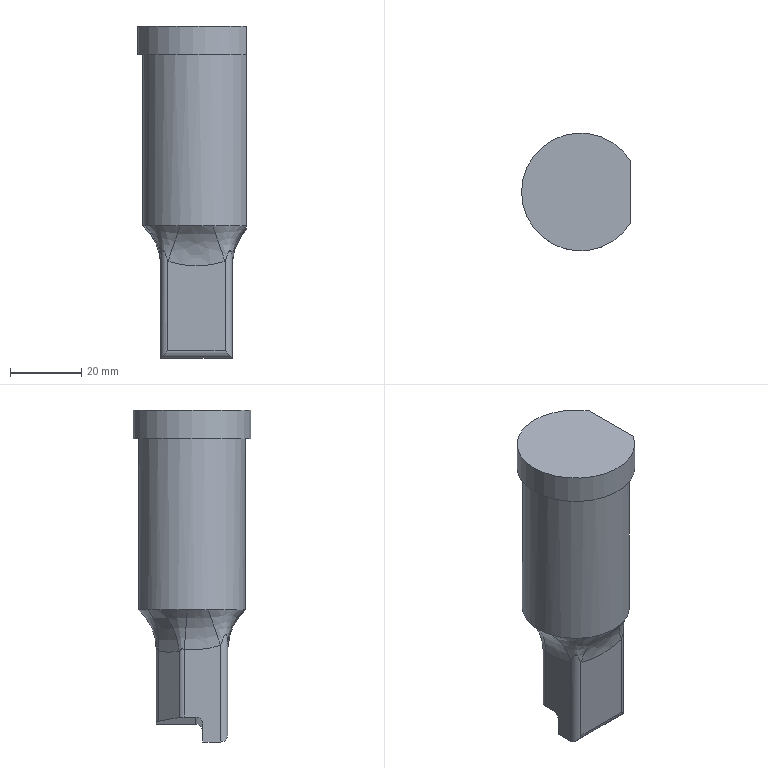Part | NX | features solid 2 | 1 solid | 34 faces | box 30.786 x 33 x 93 mm | volume 53674 mm3 | plane 13 | cylinder 11 | spline 10 | commonest cylinder face diameters 4 x9 30 x1 33 x1
STEP:
#1=CARTESIAN_POINT('',(187.901,-184.385,22.));
#2=VERTEX_POINT('',#1);
#3=CARTESIAN_POINT('',(187.901,-184.385,70.));
#4=VERTEX_POINT('',#3);
#5=CARTESIAN_POINT('',(187.901,-184.385,-33.));
#6=DIRECTION('',(0.,0.,1.));
#7=VECTOR('',#6,1000.);
#8=LINE('',#5,#7);
#9=EDGE_CURVE('',#2,#4,#8,.T.);
#10=ORIENTED_EDGE('',*,*,#9,.T.);
#11=CARTESIAN_POINT('',(187.901,-173.615,70.));
#12=VERTEX_POINT('',#11);
#13=CARTESIAN_POINT('',(173.901,-179.,70.));
#14=DIRECTION('',(0.,0.,1.));
#15=DIRECTION('',(1.,0.,0.));
#16=AXIS2_PLACEMENT_3D('',#13,#14,#15);
#17=CIRCLE('',#16,15.);
#18=EDGE_CURVE('',#4,#12,#17,.F.);
#19=ORIENTED_EDGE('',*,*,#18,.T.);
#20=CARTESIAN_POINT('',(187.901,-173.615,22.));
#21=VERTEX_POINT('',#20);
#22=CARTESIAN_POINT('',(187.901,-173.615,-33.));
#23=DIRECTION('',(0.,0.,1.));
#24=VECTOR('',#23,1000.);
#25=LINE('',#22,#24);
#26=EDGE_CURVE('',#12,#21,#25,.F.);
#27=ORIENTED_EDGE('',*,*,#26,.T.);
#28=CARTESIAN_POINT('',(178.472,-164.714,22.));
#29=VERTEX_POINT('',#28);
#30=CARTESIAN_POINT('',(173.901,-179.,22.));
#31=DIRECTION('',(0.,0.,1.));
#32=DIRECTION('',(1.,0.,0.));
#33=AXIS2_PLACEMENT_3D('',#30,#31,#32);
#34=CIRCLE('',#33,15.);
#35=EDGE_CURVE('',#21,#29,#34,.T.);
#36=ORIENTED_EDGE('',*,*,#35,.T.);
#37=CARTESIAN_POINT('',(172.603,-164.056,22.));
#38=VERTEX_POINT('',#37);
#39=CARTESIAN_POINT('',(173.901,-179.,22.));
#40=DIRECTION('',(0.,0.,1.));
#41=DIRECTION('',(1.,0.,0.));
#42=AXIS2_PLACEMENT_3D('',#39,#40,#41);
#43=CIRCLE('',#42,15.);
#44=EDGE_CURVE('',#29,#38,#43,.T.);
#45=ORIENTED_EDGE('',*,*,#44,.T.);
#46=CARTESIAN_POINT('',(165.226,-166.763,22.));
#47=VERTEX_POINT('',#46);
#48=CARTESIAN_POINT('',(173.901,-179.,22.));
#49=DIRECTION('',(0.,0.,1.));
#50=DIRECTION('',(1.,0.,0.));
#51=AXIS2_PLACEMENT_3D('',#48,#49,#50);
#52=CIRCLE('',#51,15.);
#53=EDGE_CURVE('',#38,#47,#52,.T.);
#54=ORIENTED_EDGE('',*,*,#53,.T.);
#55=CARTESIAN_POINT('',(161.663,-170.325,22.));
#56=VERTEX_POINT('',#55);
#57=CARTESIAN_POINT('',(173.901,-179.,22.));
#58=DIRECTION('',(0.,0.,1.));
#59=DIRECTION('',(1.,0.,0.));
#60=AXIS2_PLACEMENT_3D('',#57,#58,#59);
#61=CIRCLE('',#60,15.);
#62=EDGE_CURVE('',#47,#56,#61,.T.);
#63=ORIENTED_EDGE('',*,*,#62,.T.);
#64=CARTESIAN_POINT('',(158.957,-177.702,22.));
#65=VERTEX_POINT('',#64);
#66=CARTESIAN_POINT('',(173.901,-179.,22.));
#67=DIRECTION('',(0.,0.,1.));
#68=DIRECTION('',(1.,0.,0.));
#69=AXIS2_PLACEMENT_3D('',#66,#67,#68);
#70=CIRCLE('',#69,15.);
#71=EDGE_CURVE('',#56,#65,#70,.T.);
#72=ORIENTED_EDGE('',*,*,#71,.T.);
#73=CARTESIAN_POINT('',(159.614,-183.572,22.));
#74=VERTEX_POINT('',#73);
#75=CARTESIAN_POINT('',(173.901,-179.,22.));
#76=DIRECTION('',(0.,0.,1.));
#77=DIRECTION('',(1.,0.,0.));
#78=AXIS2_PLACEMENT_3D('',#75,#76,#77);
#79=CIRCLE('',#78,15.);
#80=EDGE_CURVE('',#65,#74,#79,.T.);
#81=ORIENTED_EDGE('',*,*,#80,.T.);
#82=CARTESIAN_POINT('',(169.329,-193.286,22.));
#83=VERTEX_POINT('',#82);
#84=CARTESIAN_POINT('',(173.901,-179.,22.));
#85=DIRECTION('',(0.,0.,1.));
#86=DIRECTION('',(1.,0.,0.));
#87=AXIS2_PLACEMENT_3D('',#84,#85,#86);
#88=CIRCLE('',#87,15.);
#89=EDGE_CURVE('',#74,#83,#88,.T.);
#90=ORIENTED_EDGE('',*,*,#89,.T.);
#91=CARTESIAN_POINT('',(178.472,-193.286,22.));
#92=VERTEX_POINT('',#91);
#93=CARTESIAN_POINT('',(173.901,-179.,22.));
#94=DIRECTION('',(0.,0.,1.));
#95=DIRECTION('',(1.,0.,0.));
#96=AXIS2_PLACEMENT_3D('',#93,#94,#95);
#97=CIRCLE('',#96,15.);
#98=EDGE_CURVE('',#83,#92,#97,.T.);
#99=ORIENTED_EDGE('',*,*,#98,.T.);
#100=CARTESIAN_POINT('',(173.901,-179.,22.));
#101=DIRECTION('',(0.,0.,1.));
#102=DIRECTION('',(1.,0.,0.));
#103=AXIS2_PLACEMENT_3D('',#100,#101,#102);
#104=CIRCLE('',#103,15.);
#105=EDGE_CURVE('',#92,#2,#104,.T.);
#106=ORIENTED_EDGE('',*,*,#105,.T.);
#107=EDGE_LOOP('',(#10,#19,#27,#36,#45,#54,#63,#72,#81,#90,#99,#106));
#108=FACE_BOUND('',#107,.T.);
#109=CARTESIAN_POINT('',(173.901,-179.,-33.));
#110=DIRECTION('',(0.,0.,1.));
#111=DIRECTION('',(1.,0.,0.));
#112=AXIS2_PLACEMENT_3D('',#109,#110,#111);
#113=CYLINDRICAL_SURFACE('',#112,15.);
#114=ADVANCED_FACE('',(#108),#113,.T.);
#115=CARTESIAN_POINT('',(174.401,-169.,-10.));
#116=VERTEX_POINT('',#115);
#117=CARTESIAN_POINT('',(174.901,-169.,-10.));
#118=VERTEX_POINT('',#117);
#119=CARTESIAN_POINT('',(171.729,-169.,-10.));
#120=DIRECTION('',(1.,0.,0.));
#121=VECTOR('',#120,1000.);
#122=LINE('',#119,#121);
#123=EDGE_CURVE('',#116,#118,#122,.T.);
#124=ORIENTED_EDGE('',*,*,#123,.F.);
#125=CARTESIAN_POINT('',(171.729,-169.,-9.491));
#126=VERTEX_POINT('',#125);
#127=CARTESIAN_POINT('',(174.401,-169.,-10.));
#128=DIRECTION('',(-0.9823,0.,0.1871));
#129=VECTOR('',#128,1000.);
#130=LINE('',#127,#129);
#131=EDGE_CURVE('',#116,#126,#130,.T.);
#132=ORIENTED_EDGE('',*,*,#131,.T.);
#133=CARTESIAN_POINT('',(171.729,-169.,10.905));
#134=VERTEX_POINT('',#133);
#135=CARTESIAN_POINT('',(171.729,-169.,-64.));
#136=DIRECTION('',(0.,0.,1.));
#137=VECTOR('',#136,1000.);
#138=LINE('',#135,#137);
#139=EDGE_CURVE('',#126,#134,#138,.T.);
#140=ORIENTED_EDGE('',*,*,#139,.T.);
#141=CARTESIAN_POINT('',(181.901,-169.,12.077));
#142=VERTEX_POINT('',#141);
#143=CARTESIAN_POINT('',(171.729,-169.,10.905));
#144=CARTESIAN_POINT('',(173.434,-169.,10.77));
#145=CARTESIAN_POINT('',(176.026,-169.,10.807));
#146=CARTESIAN_POINT('',(179.4,-169.,11.334));
#147=CARTESIAN_POINT('',(181.107,-169.,11.803));
#148=CARTESIAN_POINT('',(181.901,-169.,12.077));
#149=B_SPLINE_CURVE_WITH_KNOTS('',3,(#143,#144,#145,#146,#147,#148),.UNSPECIFIED.,.F.,.F.,(4,1,1,4),(0.,0.5,0.75,1.),.UNSPECIFIED.);
#150=EDGE_CURVE('',#134,#142,#149,.T.);
#151=ORIENTED_EDGE('',*,*,#150,.T.);
#152=CARTESIAN_POINT('',(181.901,-169.,-8.444));
#153=VERTEX_POINT('',#152);
#154=CARTESIAN_POINT('',(181.901,-169.,-64.));
#155=DIRECTION('',(0.,0.,1.));
#156=VECTOR('',#155,1000.);
#157=LINE('',#154,#156);
#158=EDGE_CURVE('',#153,#142,#157,.T.);
#159=ORIENTED_EDGE('',*,*,#158,.F.);
#160=CARTESIAN_POINT('',(174.901,-169.,-10.));
#161=DIRECTION('',(-0.9762,0.,-0.2169));
#162=VECTOR('',#161,1000.);
#163=LINE('',#160,#162);
#164=EDGE_CURVE('',#153,#118,#163,.T.);
#165=ORIENTED_EDGE('',*,*,#164,.T.);
#166=EDGE_LOOP('',(#124,#132,#140,#151,#159,#165));
#167=FACE_BOUND('',#166,.T.);
#168=CARTESIAN_POINT('',(171.729,-169.,-64.));
#169=DIRECTION('',(0.,-1.,0.));
#170=DIRECTION('',(1.,0.,0.));
#171=AXIS2_PLACEMENT_3D('',#168,#169,#170);
#172=PLANE('',#171);
#173=ADVANCED_FACE('',(#167),#172,.F.);
#174=CARTESIAN_POINT('',(183.901,-171.,-8.));
#175=VERTEX_POINT('',#174);
#176=CARTESIAN_POINT('',(183.901,-171.,12.077));
#177=VERTEX_POINT('',#176);
#178=CARTESIAN_POINT('',(183.901,-171.,-64.));
#179=DIRECTION('',(0.,0.,1.));
#180=VECTOR('',#179,1000.);
#181=LINE('',#178,#180);
#182=EDGE_CURVE('',#175,#177,#181,.T.);
#183=ORIENTED_EDGE('',*,*,#182,.F.);
#184=CARTESIAN_POINT('',(181.901,-171.,-8.444));
#185=DIRECTION('',(0.2169,0.,-0.9762));
#186=DIRECTION('',(0.9762,0.,0.2169));
#187=AXIS2_PLACEMENT_3D('',#184,#185,#186);
#188=ELLIPSE('',#187,2.049,2.);
#189=EDGE_CURVE('',#175,#153,#188,.F.);
#190=ORIENTED_EDGE('',*,*,#189,.T.);
#191=ORIENTED_EDGE('',*,*,#158,.T.);
#192=CARTESIAN_POINT('',(181.901,-169.,12.077));
#193=CARTESIAN_POINT('',(182.018,-169.,12.421));
#194=CARTESIAN_POINT('',(182.214,-169.021,12.984));
#195=CARTESIAN_POINT('',(182.407,-169.057,13.532));
#196=CARTESIAN_POINT('',(182.679,-169.155,14.201));
#197=CARTESIAN_POINT('',(182.775,-169.198,14.422));
#198=CARTESIAN_POINT('',(182.939,-169.289,14.732));
#199=CARTESIAN_POINT('',(183.016,-169.338,14.861));
#200=CARTESIAN_POINT('',(183.188,-169.464,15.063));
#201=CARTESIAN_POINT('',(183.318,-169.586,15.104));
#202=CARTESIAN_POINT('',(183.438,-169.714,15.062));
#203=CARTESIAN_POINT('',(183.564,-169.885,14.859));
#204=CARTESIAN_POINT('',(183.612,-169.963,14.73));
#205=CARTESIAN_POINT('',(183.703,-170.127,14.42));
#206=CARTESIAN_POINT('',(183.746,-170.222,14.199));
#207=CARTESIAN_POINT('',(183.844,-170.494,13.529));
#208=CARTESIAN_POINT('',(183.879,-170.687,12.983));
#209=CARTESIAN_POINT('',(183.901,-170.883,12.42));
#210=CARTESIAN_POINT('',(183.901,-171.,12.077));
#211=B_SPLINE_CURVE_WITH_KNOTS('',3,(#192,#193,#194,#195,#196,#197,#198,#199,#200,#201,#202,#203,#204,#205,#206,#207,#208,#209,#210),.UNSPECIFIED.,.F.,.F.,(4,1,1,1,1,1,1,1,1,1,1,1,1,1,1,1,4),(0.,0.125,0.25,0.3125,0.375,0.4062,0.4375,0.4688,0.5,0.5312,0.5625,0.5938,0.625,0.6875,0.75,0.875,1.),.UNSPECIFIED.);
#212=EDGE_CURVE('',#142,#177,#211,.T.);
#213=ORIENTED_EDGE('',*,*,#212,.T.);
#214=EDGE_LOOP('',(#183,#190,#191,#213));
#215=FACE_BOUND('',#214,.T.);
#216=CARTESIAN_POINT('',(181.901,-171.,-64.));
#217=DIRECTION('',(0.,0.,1.));
#218=DIRECTION('',(1.,0.,0.));
#219=AXIS2_PLACEMENT_3D('',#216,#217,#218);
#220=CYLINDRICAL_SURFACE('',#219,2.);
#221=ADVANCED_FACE('',(#215),#220,.T.);
#222=CARTESIAN_POINT('',(183.901,-182.,-15.));
#223=VERTEX_POINT('',#222);
#224=CARTESIAN_POINT('',(183.901,-182.,-10.049));
#225=VERTEX_POINT('',#224);
#226=CARTESIAN_POINT('',(183.901,-182.,-64.));
#227=DIRECTION('',(0.,0.,-1.));
#228=VECTOR('',#227,1000.);
#229=LINE('',#226,#228);
#230=EDGE_CURVE('',#223,#225,#229,.F.);
#231=ORIENTED_EDGE('',*,*,#230,.T.);
#232=CARTESIAN_POINT('',(183.901,-180.,-8.));
#233=VERTEX_POINT('',#232);
#234=CARTESIAN_POINT('',(183.901,-180.,-10.049));
#235=DIRECTION('',(-1.,0.,0.));
#236=DIRECTION('',(0.,0.,-1.));
#237=AXIS2_PLACEMENT_3D('',#234,#235,#236);
#238=ELLIPSE('',#237,2.049,2.);
#239=EDGE_CURVE('',#225,#233,#238,.T.);
#240=ORIENTED_EDGE('',*,*,#239,.T.);
#241=CARTESIAN_POINT('',(183.901,-171.,-8.));
#242=DIRECTION('',(0.,1.,0.));
#243=VECTOR('',#242,1000.);
#244=LINE('',#241,#243);
#245=EDGE_CURVE('',#233,#175,#244,.T.);
#246=ORIENTED_EDGE('',*,*,#245,.T.);
#247=ORIENTED_EDGE('',*,*,#182,.T.);
#248=CARTESIAN_POINT('',(183.901,-187.,12.077));
#249=VERTEX_POINT('',#248);
#250=CARTESIAN_POINT('',(183.901,-171.,12.077));
#251=CARTESIAN_POINT('',(183.901,-171.616,11.864));
#252=CARTESIAN_POINT('',(183.901,-172.879,11.493));
#253=CARTESIAN_POINT('',(183.901,-174.979,11.088));
#254=CARTESIAN_POINT('',(183.901,-176.94,10.871));
#255=CARTESIAN_POINT('',(183.901,-179.011,10.794));
#256=CARTESIAN_POINT('',(183.901,-181.061,10.872));
#257=CARTESIAN_POINT('',(183.901,-183.007,11.086));
#258=CARTESIAN_POINT('',(183.901,-185.118,11.492));
#259=CARTESIAN_POINT('',(183.901,-186.382,11.864));
#260=CARTESIAN_POINT('',(183.901,-187.,12.077));
#261=B_SPLINE_CURVE_WITH_KNOTS('',3,(#250,#251,#252,#253,#254,#255,#256,#257,#258,#259,#260),.UNSPECIFIED.,.F.,.F.,(4,1,1,1,1,1,1,1,4),(0.,0.125,0.25,0.375,0.5,0.625,0.75,0.875,1.),.UNSPECIFIED.);
#262=EDGE_CURVE('',#177,#249,#261,.T.);
#263=ORIENTED_EDGE('',*,*,#262,.T.);
#264=CARTESIAN_POINT('',(183.901,-187.,-15.));
#265=VERTEX_POINT('',#264);
#266=CARTESIAN_POINT('',(183.901,-187.,-65.));
#267=DIRECTION('',(0.,0.,1.));
#268=VECTOR('',#267,1000.);
#269=LINE('',#266,#268);
#270=EDGE_CURVE('',#265,#249,#269,.T.);
#271=ORIENTED_EDGE('',*,*,#270,.F.);
#272=CARTESIAN_POINT('',(183.901,-171.,-15.));
#273=DIRECTION('',(0.,-1.,0.));
#274=VECTOR('',#273,1000.);
#275=LINE('',#272,#274);
#276=EDGE_CURVE('',#265,#223,#275,.F.);
#277=ORIENTED_EDGE('',*,*,#276,.T.);
#278=EDGE_LOOP('',(#231,#240,#246,#247,#263,#271,#277));
#279=FACE_BOUND('',#278,.T.);
#280=CARTESIAN_POINT('',(183.901,-171.,-64.));
#281=DIRECTION('',(-1.,0.,0.));
#282=DIRECTION('',(0.,0.,1.));
#283=AXIS2_PLACEMENT_3D('',#280,#281,#282);
#284=PLANE('',#283);
#285=ADVANCED_FACE('',(#279),#284,.F.);
#286=CARTESIAN_POINT('',(181.901,-189.,-13.));
#287=VERTEX_POINT('',#286);
#288=CARTESIAN_POINT('',(181.901,-189.,12.077));
#289=VERTEX_POINT('',#288);
#290=CARTESIAN_POINT('',(181.901,-189.,-65.));
#291=DIRECTION('',(0.,0.,1.));
#292=VECTOR('',#291,1000.);
#293=LINE('',#290,#292);
#294=EDGE_CURVE('',#287,#289,#293,.T.);
#295=ORIENTED_EDGE('',*,*,#294,.F.);
#296=CARTESIAN_POINT('',(181.901,-187.,-13.));
#297=DIRECTION('',(-0.7071,0.,-0.7071));
#298=DIRECTION('',(-0.7071,0.,0.7071));
#299=AXIS2_PLACEMENT_3D('',#296,#297,#298);
#300=ELLIPSE('',#299,2.828,2.);
#301=EDGE_CURVE('',#287,#265,#300,.F.);
#302=ORIENTED_EDGE('',*,*,#301,.T.);
#303=ORIENTED_EDGE('',*,*,#270,.T.);
#304=CARTESIAN_POINT('',(183.901,-187.,12.077));
#305=CARTESIAN_POINT('',(183.901,-187.094,12.353));
#306=CARTESIAN_POINT('',(183.887,-187.284,12.904));
#307=CARTESIAN_POINT('',(183.824,-187.581,13.728));
#308=CARTESIAN_POINT('',(183.713,-187.861,14.401));
#309=CARTESIAN_POINT('',(183.569,-188.119,14.897));
#310=CARTESIAN_POINT('',(183.314,-188.438,15.193));
#311=CARTESIAN_POINT('',(183.005,-188.677,14.869));
#312=CARTESIAN_POINT('',(182.751,-188.817,14.38));
#313=CARTESIAN_POINT('',(182.476,-188.925,13.713));
#314=CARTESIAN_POINT('',(182.183,-188.987,12.899));
#315=CARTESIAN_POINT('',(181.994,-189.,12.351));
#316=CARTESIAN_POINT('',(181.901,-189.,12.077));
#317=B_SPLINE_CURVE_WITH_KNOTS('',3,(#304,#305,#306,#307,#308,#309,#310,#311,#312,#313,#314,#315,#316),.UNSPECIFIED.,.F.,.F.,(4,1,1,1,1,1,1,1,1,1,4),(0.002798,0.003672,0.004545,0.005418,0.005854,0.006291,0.006727,0.007164,0.008037,0.00891,0.009783),.UNSPECIFIED.);
#318=EDGE_CURVE('',#249,#289,#317,.T.);
#319=ORIENTED_EDGE('',*,*,#318,.T.);
#320=EDGE_LOOP('',(#295,#302,#303,#319));
#321=FACE_BOUND('',#320,.T.);
#322=CARTESIAN_POINT('',(181.901,-187.,-65.));
#323=DIRECTION('',(0.,0.,1.));
#324=DIRECTION('',(1.,0.,0.));
#325=AXIS2_PLACEMENT_3D('',#322,#323,#324);
#326=CYLINDRICAL_SURFACE('',#325,2.);
#327=ADVANCED_FACE('',(#321),#326,.T.);
#328=CARTESIAN_POINT('',(165.901,-189.,-13.));
#329=VERTEX_POINT('',#328);
#330=CARTESIAN_POINT('',(165.901,-189.,12.077));
#331=VERTEX_POINT('',#330);
#332=CARTESIAN_POINT('',(165.901,-189.,-65.));
#333=DIRECTION('',(0.,0.,1.));
#334=VECTOR('',#333,1000.);
#335=LINE('',#332,#334);
#336=EDGE_CURVE('',#329,#331,#335,.T.);
#337=ORIENTED_EDGE('',*,*,#336,.F.);
#338=CARTESIAN_POINT('',(181.901,-189.,-13.));
#339=DIRECTION('',(1.,0.,0.));
#340=VECTOR('',#339,1000.);
#341=LINE('',#338,#340);
#342=EDGE_CURVE('',#329,#287,#341,.T.);
#343=ORIENTED_EDGE('',*,*,#342,.T.);
#344=ORIENTED_EDGE('',*,*,#294,.T.);
#345=CARTESIAN_POINT('',(181.901,-189.,12.077));
#346=CARTESIAN_POINT('',(179.336,-189.,11.191));
#347=CARTESIAN_POINT('',(173.896,-189.,10.447));
#348=CARTESIAN_POINT('',(168.46,-189.,11.193));
#349=CARTESIAN_POINT('',(165.901,-189.,12.077));
#350=B_SPLINE_CURVE_WITH_KNOTS('',3,(#345,#346,#347,#348,#349),.UNSPECIFIED.,.F.,.F.,(4,1,4),(0.00601,0.01415,0.02229),.UNSPECIFIED.);
#351=EDGE_CURVE('',#289,#331,#350,.T.);
#352=ORIENTED_EDGE('',*,*,#351,.T.);
#353=EDGE_LOOP('',(#337,#343,#344,#352));
#354=FACE_BOUND('',#353,.T.);
#355=CARTESIAN_POINT('',(181.901,-189.,-65.));
#356=DIRECTION('',(0.,1.,0.));
#357=DIRECTION('',(-1.,0.,0.));
#358=AXIS2_PLACEMENT_3D('',#355,#356,#357);
#359=PLANE('',#358);
#360=ADVANCED_FACE('',(#354),#359,.F.);
#361=CARTESIAN_POINT('',(163.901,-187.,-15.));
#362=VERTEX_POINT('',#361);
#363=CARTESIAN_POINT('',(163.901,-187.,12.077));
#364=VERTEX_POINT('',#363);
#365=CARTESIAN_POINT('',(163.901,-187.,-65.));
#366=DIRECTION('',(0.,0.,1.));
#367=VECTOR('',#366,1000.);
#368=LINE('',#365,#367);
#369=EDGE_CURVE('',#362,#364,#368,.T.);
#370=ORIENTED_EDGE('',*,*,#369,.F.);
#371=CARTESIAN_POINT('',(165.901,-187.,-13.));
#372=DIRECTION('',(-0.7071,0.,0.7071));
#373=DIRECTION('',(-0.7071,0.,-0.7071));
#374=AXIS2_PLACEMENT_3D('',#371,#372,#373);
#375=ELLIPSE('',#374,2.828,2.);
#376=EDGE_CURVE('',#362,#329,#375,.T.);
#377=ORIENTED_EDGE('',*,*,#376,.T.);
#378=ORIENTED_EDGE('',*,*,#336,.T.);
#379=CARTESIAN_POINT('',(165.901,-189.,12.077));
#380=CARTESIAN_POINT('',(165.807,-189.,12.353));
#381=CARTESIAN_POINT('',(165.617,-188.987,12.904));
#382=CARTESIAN_POINT('',(165.32,-188.924,13.728));
#383=CARTESIAN_POINT('',(165.04,-188.812,14.401));
#384=CARTESIAN_POINT('',(164.782,-188.668,14.897));
#385=CARTESIAN_POINT('',(164.463,-188.413,15.193));
#386=CARTESIAN_POINT('',(164.224,-188.104,14.869));
#387=CARTESIAN_POINT('',(164.083,-187.851,14.38));
#388=CARTESIAN_POINT('',(163.976,-187.575,13.713));
#389=CARTESIAN_POINT('',(163.914,-187.282,12.899));
#390=CARTESIAN_POINT('',(163.901,-187.093,12.351));
#391=CARTESIAN_POINT('',(163.901,-187.,12.077));
#392=B_SPLINE_CURVE_WITH_KNOTS('',3,(#379,#380,#381,#382,#383,#384,#385,#386,#387,#388,#389,#390,#391),.UNSPECIFIED.,.F.,.F.,(4,1,1,1,1,1,1,1,1,1,4),(0.002798,0.003672,0.004545,0.005418,0.005854,0.006291,0.006727,0.007164,0.008037,0.00891,0.009783),.UNSPECIFIED.);
#393=EDGE_CURVE('',#331,#364,#392,.T.);
#394=ORIENTED_EDGE('',*,*,#393,.T.);
#395=EDGE_LOOP('',(#370,#377,#378,#394));
#396=FACE_BOUND('',#395,.T.);
#397=CARTESIAN_POINT('',(165.901,-187.,-65.));
#398=DIRECTION('',(0.,0.,1.));
#399=DIRECTION('',(1.,0.,0.));
#400=AXIS2_PLACEMENT_3D('',#397,#398,#399);
#401=CYLINDRICAL_SURFACE('',#400,2.);
#402=ADVANCED_FACE('',(#396),#401,.T.);
#403=CARTESIAN_POINT('',(163.901,-176.828,-8.));
#404=VERTEX_POINT('',#403);
#405=CARTESIAN_POINT('',(163.901,-176.828,10.905));
#406=VERTEX_POINT('',#405);
#407=CARTESIAN_POINT('',(163.901,-176.828,-64.));
#408=DIRECTION('',(0.,0.,1.));
#409=VECTOR('',#408,1000.);
#410=LINE('',#407,#409);
#411=EDGE_CURVE('',#404,#406,#410,.T.);
#412=ORIENTED_EDGE('',*,*,#411,.F.);
#413=CARTESIAN_POINT('',(163.901,-180.,-8.));
#414=VERTEX_POINT('',#413);
#415=CARTESIAN_POINT('',(163.901,-182.,-8.));
#416=DIRECTION('',(0.,-1.,0.));
#417=VECTOR('',#416,1000.);
#418=LINE('',#415,#417);
#419=EDGE_CURVE('',#404,#414,#418,.T.);
#420=ORIENTED_EDGE('',*,*,#419,.T.);
#421=CARTESIAN_POINT('',(163.901,-182.,-10.036));
#422=VERTEX_POINT('',#421);
#423=CARTESIAN_POINT('',(163.901,-180.,-10.036));
#424=DIRECTION('',(1.,0.,0.));
#425=DIRECTION('',(0.,0.,1.));
#426=AXIS2_PLACEMENT_3D('',#423,#424,#425);
#427=ELLIPSE('',#426,2.036,2.);
#428=EDGE_CURVE('',#414,#422,#427,.T.);
#429=ORIENTED_EDGE('',*,*,#428,.T.);
#430=CARTESIAN_POINT('',(163.901,-182.,-15.));
#431=VERTEX_POINT('',#430);
#432=CARTESIAN_POINT('',(163.901,-182.,-64.));
#433=DIRECTION('',(0.,0.,1.));
#434=VECTOR('',#433,1000.);
#435=LINE('',#432,#434);
#436=EDGE_CURVE('',#422,#431,#435,.F.);
#437=ORIENTED_EDGE('',*,*,#436,.T.);
#438=CARTESIAN_POINT('',(163.901,-187.,-15.));
#439=DIRECTION('',(0.,1.,0.));
#440=VECTOR('',#439,1000.);
#441=LINE('',#438,#440);
#442=EDGE_CURVE('',#431,#362,#441,.F.);
#443=ORIENTED_EDGE('',*,*,#442,.T.);
#444=ORIENTED_EDGE('',*,*,#369,.T.);
#445=CARTESIAN_POINT('',(163.901,-187.,12.077));
#446=CARTESIAN_POINT('',(163.901,-185.422,11.532));
#447=CARTESIAN_POINT('',(163.901,-181.971,10.809));
#448=CARTESIAN_POINT('',(163.901,-178.535,10.77));
#449=CARTESIAN_POINT('',(163.901,-176.828,10.905));
#450=B_SPLINE_CURVE_WITH_KNOTS('',3,(#445,#446,#447,#448,#449),.UNSPECIFIED.,.F.,.F.,(4,1,4),(0.,0.5,1.),.UNSPECIFIED.);
#451=EDGE_CURVE('',#364,#406,#450,.T.);
#452=ORIENTED_EDGE('',*,*,#451,.T.);
#453=EDGE_LOOP('',(#412,#420,#429,#437,#443,#444,#452));
#454=FACE_BOUND('',#453,.T.);
#455=CARTESIAN_POINT('',(163.901,-187.,-64.));
#456=DIRECTION('',(1.,0.,0.));
#457=DIRECTION('',(0.,0.,-1.));
#458=AXIS2_PLACEMENT_3D('',#455,#456,#457);
#459=PLANE('',#458);
#460=ADVANCED_FACE('',(#454),#459,.F.);
#461=CARTESIAN_POINT('',(164.486,-175.414,-8.112));
#462=VERTEX_POINT('',#461);
#463=CARTESIAN_POINT('',(164.486,-175.414,10.425));
#464=VERTEX_POINT('',#463);
#465=CARTESIAN_POINT('',(164.486,-175.414,-64.));
#466=DIRECTION('',(0.,0.,1.));
#467=VECTOR('',#466,1000.);
#468=LINE('',#465,#467);
#469=EDGE_CURVE('',#462,#464,#468,.T.);
#470=ORIENTED_EDGE('',*,*,#469,.F.);
#471=CARTESIAN_POINT('',(165.901,-176.828,-8.381));
#472=DIRECTION('',(-0.1871,0.,-0.9823));
#473=DIRECTION('',(-0.9823,0.,0.1871));
#474=AXIS2_PLACEMENT_3D('',#471,#472,#473);
#475=ELLIPSE('',#474,2.036,2.);
#476=EDGE_CURVE('',#462,#404,#475,.F.);
#477=ORIENTED_EDGE('',*,*,#476,.T.);
#478=ORIENTED_EDGE('',*,*,#411,.T.);
#479=CARTESIAN_POINT('',(163.901,-176.828,10.905));
#480=CARTESIAN_POINT('',(163.901,-176.685,11.001));
#481=CARTESIAN_POINT('',(163.922,-176.424,11.125));
#482=CARTESIAN_POINT('',(164.091,-175.944,11.028));
#483=CARTESIAN_POINT('',(164.24,-175.701,10.818));
#484=CARTESIAN_POINT('',(164.398,-175.502,10.572));
#485=CARTESIAN_POINT('',(164.486,-175.414,10.425));
#486=B_SPLINE_CURVE_WITH_KNOTS('',3,(#479,#480,#481,#482,#483,#484,#485),.UNSPECIFIED.,.F.,.F.,(4,1,1,1,4),(0.,0.25,0.5,0.75,1.),.UNSPECIFIED.);
#487=EDGE_CURVE('',#406,#464,#486,.T.);
#488=ORIENTED_EDGE('',*,*,#487,.T.);
#489=EDGE_LOOP('',(#470,#477,#478,#488));
#490=FACE_BOUND('',#489,.T.);
#491=CARTESIAN_POINT('',(165.901,-176.828,-64.));
#492=DIRECTION('',(0.,0.,1.));
#493=DIRECTION('',(1.,0.,0.));
#494=AXIS2_PLACEMENT_3D('',#491,#492,#493);
#495=CYLINDRICAL_SURFACE('',#494,2.);
#496=ADVANCED_FACE('',(#490),#495,.T.);
#497=CARTESIAN_POINT('',(170.315,-169.586,-9.222));
#498=VERTEX_POINT('',#497);
#499=CARTESIAN_POINT('',(170.315,-169.586,10.425));
#500=VERTEX_POINT('',#499);
#501=CARTESIAN_POINT('',(170.315,-169.586,-64.));
#502=DIRECTION('',(0.,0.,1.));
#503=VECTOR('',#502,1000.);
#504=LINE('',#501,#503);
#505=EDGE_CURVE('',#498,#500,#504,.T.);
#506=ORIENTED_EDGE('',*,*,#505,.F.);
#507=CARTESIAN_POINT('',(180.238,-159.663,-11.112));
#508=DIRECTION('',(-0.7008,-0.7008,0.1335));
#509=VECTOR('',#508,1000.);
#510=LINE('',#507,#509);
#511=EDGE_CURVE('',#498,#462,#510,.T.);
#512=ORIENTED_EDGE('',*,*,#511,.T.);
#513=ORIENTED_EDGE('',*,*,#469,.T.);
#514=CARTESIAN_POINT('',(164.486,-175.414,10.425));
#515=CARTESIAN_POINT('',(166.386,-173.515,10.054));
#516=CARTESIAN_POINT('',(168.418,-171.483,10.054));
#517=CARTESIAN_POINT('',(170.315,-169.586,10.425));
#518=B_SPLINE_CURVE_WITH_KNOTS('',3,(#514,#515,#516,#517),.UNSPECIFIED.,.F.,.F.,(4,4),(0.,1.),.UNSPECIFIED.);
#519=EDGE_CURVE('',#464,#500,#518,.T.);
#520=ORIENTED_EDGE('',*,*,#519,.T.);
#521=EDGE_LOOP('',(#506,#512,#513,#520));
#522=FACE_BOUND('',#521,.T.);
#523=CARTESIAN_POINT('',(164.486,-175.414,-64.));
#524=DIRECTION('',(0.7071,-0.7071,0.));
#525=DIRECTION('',(0.7071,0.7071,0.));
#526=AXIS2_PLACEMENT_3D('',#523,#524,#525);
#527=PLANE('',#526);
#528=ADVANCED_FACE('',(#522),#527,.F.);
#529=ORIENTED_EDGE('',*,*,#139,.F.);
#530=CARTESIAN_POINT('',(171.729,-171.,-9.491));
#531=DIRECTION('',(-0.1871,0.,-0.9823));
#532=DIRECTION('',(-0.9823,0.,0.1871));
#533=AXIS2_PLACEMENT_3D('',#530,#531,#532);
#534=ELLIPSE('',#533,2.036,2.);
#535=EDGE_CURVE('',#126,#498,#534,.F.);
#536=ORIENTED_EDGE('',*,*,#535,.T.);
#537=ORIENTED_EDGE('',*,*,#505,.T.);
#538=CARTESIAN_POINT('',(170.315,-169.586,10.425));
#539=CARTESIAN_POINT('',(170.403,-169.497,10.573));
#540=CARTESIAN_POINT('',(170.602,-169.339,10.819));
#541=CARTESIAN_POINT('',(170.847,-169.189,11.029));
#542=CARTESIAN_POINT('',(171.325,-169.022,11.125));
#543=CARTESIAN_POINT('',(171.586,-169.,11.));
#544=CARTESIAN_POINT('',(171.729,-169.,10.905));
#545=B_SPLINE_CURVE_WITH_KNOTS('',3,(#538,#539,#540,#541,#542,#543,#544),.UNSPECIFIED.,.F.,.F.,(4,1,1,1,4),(0.,0.25,0.5,0.75,1.),.UNSPECIFIED.);
#546=EDGE_CURVE('',#500,#134,#545,.T.);
#547=ORIENTED_EDGE('',*,*,#546,.T.);
#548=EDGE_LOOP('',(#529,#536,#537,#547));
#549=FACE_BOUND('',#548,.T.);
#550=CARTESIAN_POINT('',(171.729,-171.,-64.));
#551=DIRECTION('',(0.,0.,1.));
#552=DIRECTION('',(1.,0.,0.));
#553=AXIS2_PLACEMENT_3D('',#550,#551,#552);
#554=CYLINDRICAL_SURFACE('',#553,2.);
#555=ADVANCED_FACE('',(#549),#554,.T.);
#556=CARTESIAN_POINT('',(174.901,-180.,-10.));
#557=VERTEX_POINT('',#556);
#558=CARTESIAN_POINT('',(174.901,-182.,-10.));
#559=DIRECTION('',(0.,-1.,0.));
#560=VECTOR('',#559,1000.);
#561=LINE('',#558,#560);
#562=EDGE_CURVE('',#118,#557,#561,.T.);
#563=ORIENTED_EDGE('',*,*,#562,.T.);
#564=CARTESIAN_POINT('',(174.401,-180.,-10.));
#565=VERTEX_POINT('',#564);
#566=CARTESIAN_POINT('',(174.401,-180.,-10.));
#567=DIRECTION('',(1.,0.,0.));
#568=VECTOR('',#567,1000.);
#569=LINE('',#566,#568);
#570=EDGE_CURVE('',#557,#565,#569,.F.);
#571=ORIENTED_EDGE('',*,*,#570,.T.);
#572=CARTESIAN_POINT('',(174.401,-176.828,-10.));
#573=DIRECTION('',(0.,1.,0.));
#574=VECTOR('',#573,1000.);
#575=LINE('',#572,#574);
#576=EDGE_CURVE('',#565,#116,#575,.T.);
#577=ORIENTED_EDGE('',*,*,#576,.T.);
#578=ORIENTED_EDGE('',*,*,#123,.T.);
#579=EDGE_LOOP('',(#563,#571,#577,#578));
#580=FACE_BOUND('',#579,.T.);
#581=CARTESIAN_POINT('',(164.065,-153.614,-10.));
#582=DIRECTION('',(0.,0.,-1.));
#583=DIRECTION('',(-1.,0.,0.));
#584=AXIS2_PLACEMENT_3D('',#581,#582,#583);
#585=PLANE('',#584);
#586=ADVANCED_FACE('',(#580),#585,.T.);
#587=CARTESIAN_POINT('',(187.901,-187.732,78.));
#588=VERTEX_POINT('',#587);
#589=CARTESIAN_POINT('',(187.901,-187.732,70.));
#590=VERTEX_POINT('',#589);
#591=CARTESIAN_POINT('',(187.901,-187.732,70.));
#592=DIRECTION('',(0.,0.,1.));
#593=VECTOR('',#592,1000.);
#594=LINE('',#591,#593);
#595=EDGE_CURVE('',#588,#590,#594,.F.);
#596=ORIENTED_EDGE('',*,*,#595,.F.);
#597=CARTESIAN_POINT('',(187.901,-170.268,78.));
#598=VERTEX_POINT('',#597);
#599=CARTESIAN_POINT('',(173.901,-179.,78.));
#600=DIRECTION('',(0.,0.,-1.));
#601=DIRECTION('',(-1.,0.,0.));
#602=AXIS2_PLACEMENT_3D('',#599,#600,#601);
#603=CIRCLE('',#602,16.5);
#604=EDGE_CURVE('',#588,#598,#603,.T.);
#605=ORIENTED_EDGE('',*,*,#604,.T.);
#606=CARTESIAN_POINT('',(187.901,-170.268,70.));
#607=VERTEX_POINT('',#606);
#608=CARTESIAN_POINT('',(187.901,-170.268,70.));
#609=DIRECTION('',(0.,0.,1.));
#610=VECTOR('',#609,1000.);
#611=LINE('',#608,#610);
#612=EDGE_CURVE('',#607,#598,#611,.T.);
#613=ORIENTED_EDGE('',*,*,#612,.F.);
#614=CARTESIAN_POINT('',(173.901,-179.,70.));
#615=DIRECTION('',(0.,0.,1.));
#616=DIRECTION('',(1.,0.,0.));
#617=AXIS2_PLACEMENT_3D('',#614,#615,#616);
#618=CIRCLE('',#617,16.5);
#619=EDGE_CURVE('',#590,#607,#618,.F.);
#620=ORIENTED_EDGE('',*,*,#619,.F.);
#621=EDGE_LOOP('',(#596,#605,#613,#620));
#622=FACE_BOUND('',#621,.T.);
#623=CARTESIAN_POINT('',(173.901,-179.,70.));
#624=DIRECTION('',(0.,0.,1.));
#625=DIRECTION('',(1.,0.,0.));
#626=AXIS2_PLACEMENT_3D('',#623,#624,#625);
#627=CYLINDRICAL_SURFACE('',#626,16.5);
#628=ADVANCED_FACE('',(#622),#627,.T.);
#629=ORIENTED_EDGE('',*,*,#619,.T.);
#630=CARTESIAN_POINT('',(187.901,-179.,70.));
#631=DIRECTION('',(0.,-1.,0.));
#632=VECTOR('',#631,1000.);
#633=LINE('',#630,#632);
#634=EDGE_CURVE('',#12,#607,#633,.F.);
#635=ORIENTED_EDGE('',*,*,#634,.F.);
#636=ORIENTED_EDGE('',*,*,#18,.F.);
#637=CARTESIAN_POINT('',(187.901,-179.,70.));
#638=DIRECTION('',(0.,-1.,0.));
#639=VECTOR('',#638,1000.);
#640=LINE('',#637,#639);
#641=EDGE_CURVE('',#590,#4,#640,.F.);
#642=ORIENTED_EDGE('',*,*,#641,.F.);
#643=EDGE_LOOP('',(#629,#635,#636,#642));
#644=FACE_BOUND('',#643,.T.);
#645=CARTESIAN_POINT('',(173.901,-179.,70.));
#646=DIRECTION('',(0.,0.,1.));
#647=DIRECTION('',(1.,0.,0.));
#648=AXIS2_PLACEMENT_3D('',#645,#646,#647);
#649=PLANE('',#648);
#650=ADVANCED_FACE('',(#644),#649,.F.);
#651=ORIENTED_EDGE('',*,*,#604,.F.);
#652=CARTESIAN_POINT('',(187.901,-140.,78.));
#653=DIRECTION('',(0.,1.,0.));
#654=VECTOR('',#653,1000.);
#655=LINE('',#652,#654);
#656=EDGE_CURVE('',#588,#598,#655,.T.);
#657=ORIENTED_EDGE('',*,*,#656,.T.);
#658=EDGE_LOOP('',(#651,#657));
#659=FACE_BOUND('',#658,.T.);
#660=CARTESIAN_POINT('',(149.,-140.,78.));
#661=DIRECTION('',(0.,0.,-1.));
#662=DIRECTION('',(-1.,0.,0.));
#663=AXIS2_PLACEMENT_3D('',#660,#661,#662);
#664=PLANE('',#663);
#665=ADVANCED_FACE('',(#659),#664,.F.);
#666=CARTESIAN_POINT('',(159.708,-158.979,10.425));
#667=DIRECTION('',(0.7004,0.7004,0.1371));
#668=DIRECTION('',(-0.7071,0.7071,0.));
#669=AXIS2_PLACEMENT_3D('',#666,#667,#668);
#670=CIRCLE('',#669,15.);
#671=EDGE_CURVE('',#47,#500,#670,.T.);
#672=ORIENTED_EDGE('',*,*,#671,.T.);
#673=ORIENTED_EDGE('',*,*,#519,.F.);
#674=CARTESIAN_POINT('',(153.88,-164.808,10.425));
#675=DIRECTION('',(0.7004,0.7004,-0.1371));
#676=DIRECTION('',(-0.7071,0.7071,0.));
#677=AXIS2_PLACEMENT_3D('',#674,#675,#676);
#678=CIRCLE('',#677,15.);
#679=EDGE_CURVE('',#56,#464,#678,.T.);
#680=ORIENTED_EDGE('',*,*,#679,.F.);
#681=ORIENTED_EDGE('',*,*,#62,.F.);
#682=EDGE_LOOP('',(#672,#673,#680,#681));
#683=FACE_BOUND('',#682,.T.);
#684=CARTESIAN_POINT('',(165.226,-166.763,22.));
#685=CARTESIAN_POINT('',(169.618,-170.282,17.539));
#686=CARTESIAN_POINT('',(170.315,-169.586,10.425));
#687=CARTESIAN_POINT('',(163.885,-167.713,22.));
#688=CARTESIAN_POINT('',(168.155,-171.746,17.474));
#689=CARTESIAN_POINT('',(168.386,-171.514,10.048));
#690=CARTESIAN_POINT('',(162.619,-168.978,22.));
#691=CARTESIAN_POINT('',(166.654,-173.247,17.474));
#692=CARTESIAN_POINT('',(166.425,-173.476,10.046));
#693=CARTESIAN_POINT('',(161.663,-170.325,22.));
#694=CARTESIAN_POINT('',(165.183,-174.718,17.539));
#695=CARTESIAN_POINT('',(164.486,-175.414,10.425));
#696=(BOUNDED_SURFACE()B_SPLINE_SURFACE(3,2,((#684,#685,#686),(#687,#688,#689),(#690,#691,#692),(#693,#694,#695)),.UNSPECIFIED.,.F.,.F.,.F.)B_SPLINE_SURFACE_WITH_KNOTS((4,4),(3,3),(0.01944,0.02772),(0.,1.),.PIECEWISE_BEZIER_KNOTS.)GEOMETRIC_REPRESENTATION_ITEM()RATIONAL_B_SPLINE_SURFACE(((1.,0.902,1.),(1.,0.8969,1.),(1.,0.8968,1.),(1.,0.902,1.)))REPRESENTATION_ITEM('')SURFACE());
#697=ADVANCED_FACE('',(#683),#696,.F.);
#698=ORIENTED_EDGE('',*,*,#679,.T.);
#699=ORIENTED_EDGE('',*,*,#487,.F.);
#700=CARTESIAN_POINT('',(148.901,-176.828,10.905));
#701=DIRECTION('',(0.,0.9969,0.07848));
#702=DIRECTION('',(0.,-0.07848,0.9969));
#703=AXIS2_PLACEMENT_3D('',#700,#701,#702);
#704=CIRCLE('',#703,15.);
#705=EDGE_CURVE('',#65,#406,#704,.T.);
#706=ORIENTED_EDGE('',*,*,#705,.F.);
#707=ORIENTED_EDGE('',*,*,#71,.F.);
#708=EDGE_LOOP('',(#698,#699,#706,#707));
#709=FACE_BOUND('',#708,.T.);
#710=CARTESIAN_POINT('',(161.663,-170.325,22.));
#711=CARTESIAN_POINT('',(165.183,-174.718,17.539));
#712=CARTESIAN_POINT('',(164.486,-175.414,10.425));
#713=CARTESIAN_POINT('',(160.888,-171.419,22.));
#714=CARTESIAN_POINT('',(164.756,-174.964,17.531));
#715=CARTESIAN_POINT('',(164.301,-175.599,10.733));
#716=CARTESIAN_POINT('',(159.652,-173.777,22.));
#717=CARTESIAN_POINT('',(164.011,-175.745,17.568));
#718=CARTESIAN_POINT('',(164.005,-176.041,11.179));
#719=CARTESIAN_POINT('',(159.071,-176.388,22.));
#720=CARTESIAN_POINT('',(163.833,-176.843,17.556));
#721=CARTESIAN_POINT('',(163.901,-176.568,11.079));
#722=CARTESIAN_POINT('',(158.957,-177.702,22.));
#723=CARTESIAN_POINT('',(163.901,-177.351,17.547));
#724=CARTESIAN_POINT('',(163.901,-176.828,10.905));
#725=(BOUNDED_SURFACE()B_SPLINE_SURFACE(3,2,((#710,#711,#712),(#713,#714,#715),(#716,#717,#718),(#719,#720,#721),(#722,#723,#724)),.UNSPECIFIED.,.F.,.F.,.F.)B_SPLINE_SURFACE_WITH_KNOTS((4,1,4),(3,3),(0.05052,0.05717,0.06382),(0.,1.),.UNSPECIFIED.)GEOMETRIC_REPRESENTATION_ITEM()RATIONAL_B_SPLINE_SURFACE(((1.,0.902,1.),(1.,0.91,1.),(1.,0.9203,1.),(1.,0.9181,1.),(1.,0.9139,1.)))REPRESENTATION_ITEM('')SURFACE());
#726=ADVANCED_FACE('',(#709),#725,.F.);
#727=ORIENTED_EDGE('',*,*,#671,.F.);
#728=ORIENTED_EDGE('',*,*,#53,.F.);
#729=CARTESIAN_POINT('',(171.729,-154.,10.905));
#730=DIRECTION('',(0.9969,0.,-0.07848));
#731=DIRECTION('',(-0.07848,0.,-0.9969));
#732=AXIS2_PLACEMENT_3D('',#729,#730,#731);
#733=CIRCLE('',#732,15.);
#734=EDGE_CURVE('',#38,#134,#733,.T.);
#735=ORIENTED_EDGE('',*,*,#734,.T.);
#736=ORIENTED_EDGE('',*,*,#546,.F.);
#737=EDGE_LOOP('',(#727,#728,#735,#736));
#738=FACE_BOUND('',#737,.T.);
#739=CARTESIAN_POINT('',(172.603,-164.056,22.));
#740=CARTESIAN_POINT('',(172.252,-169.,17.547));
#741=CARTESIAN_POINT('',(171.729,-169.,10.905));
#742=CARTESIAN_POINT('',(171.291,-164.17,22.));
#743=CARTESIAN_POINT('',(171.745,-168.932,17.556));
#744=CARTESIAN_POINT('',(171.469,-169.,11.079));
#745=CARTESIAN_POINT('',(168.669,-164.755,22.));
#746=CARTESIAN_POINT('',(170.643,-169.112,17.568));
#747=CARTESIAN_POINT('',(170.94,-169.105,11.179));
#748=CARTESIAN_POINT('',(166.322,-165.986,22.));
#749=CARTESIAN_POINT('',(169.865,-169.854,17.531));
#750=CARTESIAN_POINT('',(170.5,-169.4,10.734));
#751=CARTESIAN_POINT('',(165.226,-166.763,22.));
#752=CARTESIAN_POINT('',(169.618,-170.282,17.539));
#753=CARTESIAN_POINT('',(170.315,-169.586,10.425));
#754=(BOUNDED_SURFACE()B_SPLINE_SURFACE(3,2,((#739,#740,#741),(#742,#743,#744),(#745,#746,#747),(#748,#749,#750),(#751,#752,#753)),.UNSPECIFIED.,.F.,.F.,.F.)B_SPLINE_SURFACE_WITH_KNOTS((4,1,4),(3,3),(0.0481,0.05477,0.06143),(0.,1.),.UNSPECIFIED.)GEOMETRIC_REPRESENTATION_ITEM()RATIONAL_B_SPLINE_SURFACE(((1.,0.9139,1.),(1.,0.918,1.),(1.,0.9203,1.),(1.,0.91,1.),(1.,0.902,1.)))REPRESENTATION_ITEM('')SURFACE());
#755=ADVANCED_FACE('',(#738),#754,.F.);
#756=ORIENTED_EDGE('',*,*,#705,.T.);
#757=ORIENTED_EDGE('',*,*,#451,.F.);
#758=CARTESIAN_POINT('',(148.901,-187.,12.077));
#759=DIRECTION('',(0.,0.9452,-0.3266));
#760=DIRECTION('',(0.,0.3266,0.9452));
#761=AXIS2_PLACEMENT_3D('',#758,#759,#760);
#762=CIRCLE('',#761,15.);
#763=EDGE_CURVE('',#74,#364,#762,.T.);
#764=ORIENTED_EDGE('',*,*,#763,.F.);
#765=ORIENTED_EDGE('',*,*,#80,.F.);
#766=EDGE_LOOP('',(#756,#757,#764,#765));
#767=FACE_BOUND('',#766,.T.);
#768=CARTESIAN_POINT('',(158.957,-177.702,22.));
#769=CARTESIAN_POINT('',(163.901,-177.351,17.547));
#770=CARTESIAN_POINT('',(163.901,-176.828,10.905));
#771=CARTESIAN_POINT('',(158.781,-179.726,22.));
#772=CARTESIAN_POINT('',(163.901,-179.945,17.485));
#773=CARTESIAN_POINT('',(163.901,-180.239,10.636));
#774=CARTESIAN_POINT('',(159.075,-181.886,22.));
#775=CARTESIAN_POINT('',(163.901,-182.595,17.515));
#776=CARTESIAN_POINT('',(163.901,-183.748,10.954));
#777=CARTESIAN_POINT('',(159.614,-183.572,22.));
#778=CARTESIAN_POINT('',(163.901,-185.,17.866));
#779=CARTESIAN_POINT('',(163.901,-187.,12.077));
#780=(BOUNDED_SURFACE()B_SPLINE_SURFACE(3,2,((#768,#769,#770),(#771,#772,#773),(#774,#775,#776),(#777,#778,#779)),.UNSPECIFIED.,.F.,.F.,.F.)B_SPLINE_SURFACE_WITH_KNOTS((4,4),(3,3),(0.01989,0.03021),(0.,1.),.PIECEWISE_BEZIER_KNOTS.)GEOMETRIC_REPRESENTATION_ITEM()RATIONAL_B_SPLINE_SURFACE(((1.,0.9139,1.),(1.,0.9107,1.),(1.,0.9161,1.),(1.,0.9258,1.)))REPRESENTATION_ITEM('')SURFACE());
#781=ADVANCED_FACE('',(#767),#780,.F.);
#782=ORIENTED_EDGE('',*,*,#734,.F.);
#783=ORIENTED_EDGE('',*,*,#44,.F.);
#784=CARTESIAN_POINT('',(181.901,-154.,12.077));
#785=DIRECTION('',(0.9452,0.,0.3266));
#786=DIRECTION('',(0.3266,0.,-0.9452));
#787=AXIS2_PLACEMENT_3D('',#784,#785,#786);
#788=CIRCLE('',#787,15.);
#789=EDGE_CURVE('',#142,#29,#788,.F.);
#790=ORIENTED_EDGE('',*,*,#789,.F.);
#791=ORIENTED_EDGE('',*,*,#150,.F.);
#792=EDGE_LOOP('',(#782,#783,#790,#791));
#793=FACE_BOUND('',#792,.T.);
#794=CARTESIAN_POINT('',(178.472,-164.714,22.));
#795=CARTESIAN_POINT('',(179.901,-169.,17.866));
#796=CARTESIAN_POINT('',(181.901,-169.,12.077));
#797=CARTESIAN_POINT('',(177.631,-164.444,22.));
#798=CARTESIAN_POINT('',(178.706,-169.,17.692));
#799=CARTESIAN_POINT('',(180.278,-169.,11.516));
#800=CARTESIAN_POINT('',(175.702,-164.002,22.));
#801=CARTESIAN_POINT('',(176.148,-169.,17.523));
#802=CARTESIAN_POINT('',(176.859,-169.,10.814));
#803=CARTESIAN_POINT('',(173.622,-163.968,22.));
#804=CARTESIAN_POINT('',(173.556,-169.,17.516));
#805=CARTESIAN_POINT('',(173.447,-169.,10.769));
#806=CARTESIAN_POINT('',(172.603,-164.056,22.));
#807=CARTESIAN_POINT('',(172.252,-169.,17.547));
#808=CARTESIAN_POINT('',(171.729,-169.,10.905));
#809=(BOUNDED_SURFACE()B_SPLINE_SURFACE(3,2,((#794,#795,#796),(#797,#798,#799),(#800,#801,#802),(#803,#804,#805),(#806,#807,#808)),.UNSPECIFIED.,.F.,.F.,.F.)B_SPLINE_SURFACE_WITH_KNOTS((4,1,4),(3,3),(0.01394,0.0191,0.02426),(0.,1.),.UNSPECIFIED.)GEOMETRIC_REPRESENTATION_ITEM()RATIONAL_B_SPLINE_SURFACE(((1.,0.9258,1.),(1.,0.921,1.),(1.,0.9129,1.),(1.,0.9123,1.),(1.,0.9139,1.)))REPRESENTATION_ITEM('')SURFACE());
#810=ADVANCED_FACE('',(#793),#809,.F.);
#811=ORIENTED_EDGE('',*,*,#763,.T.);
#812=ORIENTED_EDGE('',*,*,#393,.F.);
#813=CARTESIAN_POINT('',(165.901,-204.,12.077));
#814=DIRECTION('',(-0.9452,0.,0.3266));
#815=DIRECTION('',(0.3266,0.,0.9452));
#816=AXIS2_PLACEMENT_3D('',#813,#814,#815);
#817=CIRCLE('',#816,15.);
#818=EDGE_CURVE('',#83,#331,#817,.T.);
#819=ORIENTED_EDGE('',*,*,#818,.F.);
#820=ORIENTED_EDGE('',*,*,#89,.F.);
#821=EDGE_LOOP('',(#811,#812,#819,#820));
#822=FACE_BOUND('',#821,.T.);
#823=CARTESIAN_POINT('',(159.614,-183.572,22.));
#824=CARTESIAN_POINT('',(163.901,-185.,17.866));
#825=CARTESIAN_POINT('',(163.901,-187.,12.077));
#826=CARTESIAN_POINT('',(159.973,-184.692,22.));
#827=CARTESIAN_POINT('',(163.65,-185.496,17.996));
#828=CARTESIAN_POINT('',(163.901,-187.254,12.824));
#829=CARTESIAN_POINT('',(160.932,-186.815,22.));
#830=CARTESIAN_POINT('',(163.424,-186.711,18.434));
#831=CARTESIAN_POINT('',(163.995,-187.762,14.307));
#832=CARTESIAN_POINT('',(163.189,-189.715,22.));
#833=CARTESIAN_POINT('',(164.33,-188.572,18.907));
#834=CARTESIAN_POINT('',(164.447,-188.455,15.48));
#835=CARTESIAN_POINT('',(166.07,-191.959,22.));
#836=CARTESIAN_POINT('',(166.18,-189.475,18.436));
#837=CARTESIAN_POINT('',(165.135,-188.904,14.315));
#838=CARTESIAN_POINT('',(168.209,-192.928,22.));
#839=CARTESIAN_POINT('',(167.405,-189.25,17.996));
#840=CARTESIAN_POINT('',(165.646,-189.,12.824));
#841=CARTESIAN_POINT('',(169.329,-193.286,22.));
#842=CARTESIAN_POINT('',(167.901,-189.,17.866));
#843=CARTESIAN_POINT('',(165.901,-189.,12.077));
#844=(BOUNDED_SURFACE()B_SPLINE_SURFACE(3,2,((#823,#824,#825),(#826,#827,#828),(#829,#830,#831),(#832,#833,#834),(#835,#836,#837),(#838,#839,#840),(#841,#842,#843)),.UNSPECIFIED.,.F.,.F.,.F.)B_SPLINE_SURFACE_WITH_KNOTS((4,1,1,1,4),(3,3),(0.04172,0.04855,0.05538,0.06222,0.06905),(0.,1.),.UNSPECIFIED.)GEOMETRIC_REPRESENTATION_ITEM()RATIONAL_B_SPLINE_SURFACE(((1.,0.9258,1.),(1.,0.9401,1.),(1.,0.9628,1.),(1.,0.9758,1.),(1.,0.9629,1.),(1.,0.9401,1.),(1.,0.9258,1.)))REPRESENTATION_ITEM('')SURFACE());
#845=ADVANCED_FACE('',(#822),#844,.F.);
#846=ORIENTED_EDGE('',*,*,#35,.F.);
#847=CARTESIAN_POINT('',(187.901,-174.33,21.716));
#848=VERTEX_POINT('',#847);
#849=CARTESIAN_POINT('',(187.901,-173.615,22.));
#850=CARTESIAN_POINT('',(187.901,-173.849,21.895));
#851=CARTESIAN_POINT('',(187.901,-174.088,21.8));
#852=CARTESIAN_POINT('',(187.901,-174.33,21.716));
#853=B_SPLINE_CURVE_WITH_KNOTS('',3,(#849,#850,#851,#852),.UNSPECIFIED.,.F.,.F.,(4,4),(0.,0.0007697),.UNSPECIFIED.);
#854=EDGE_CURVE('',#21,#848,#853,.T.);
#855=ORIENTED_EDGE('',*,*,#854,.T.);
#856=CARTESIAN_POINT('',(198.901,-171.,12.077));
#857=DIRECTION('',(0.,-0.9452,-0.3266));
#858=DIRECTION('',(0.,0.3266,-0.9452));
#859=AXIS2_PLACEMENT_3D('',#856,#857,#858);
#860=CIRCLE('',#859,15.);
#861=EDGE_CURVE('',#177,#848,#860,.F.);
#862=ORIENTED_EDGE('',*,*,#861,.F.);
#863=ORIENTED_EDGE('',*,*,#212,.F.);
#864=ORIENTED_EDGE('',*,*,#789,.T.);
#865=EDGE_LOOP('',(#846,#855,#862,#863,#864));
#866=FACE_BOUND('',#865,.T.);
#867=CARTESIAN_POINT('',(188.187,-174.428,22.));
#868=CARTESIAN_POINT('',(183.901,-173.,17.866));
#869=CARTESIAN_POINT('',(183.901,-171.,12.077));
#870=CARTESIAN_POINT('',(187.828,-173.308,22.));
#871=CARTESIAN_POINT('',(184.151,-172.504,17.996));
#872=CARTESIAN_POINT('',(183.901,-170.746,12.824));
#873=CARTESIAN_POINT('',(186.869,-171.185,22.));
#874=CARTESIAN_POINT('',(184.377,-171.289,18.434));
#875=CARTESIAN_POINT('',(183.806,-170.238,14.307));
#876=CARTESIAN_POINT('',(184.612,-168.285,22.));
#877=CARTESIAN_POINT('',(183.471,-169.428,18.907));
#878=CARTESIAN_POINT('',(183.354,-169.545,15.48));
#879=CARTESIAN_POINT('',(181.731,-166.041,22.));
#880=CARTESIAN_POINT('',(181.621,-168.525,18.436));
#881=CARTESIAN_POINT('',(182.667,-169.096,14.315));
#882=CARTESIAN_POINT('',(179.593,-165.072,22.));
#883=CARTESIAN_POINT('',(180.396,-168.75,17.996));
#884=CARTESIAN_POINT('',(182.155,-169.,12.824));
#885=CARTESIAN_POINT('',(178.472,-164.714,22.));
#886=CARTESIAN_POINT('',(179.901,-169.,17.866));
#887=CARTESIAN_POINT('',(181.901,-169.,12.077));
#888=(BOUNDED_SURFACE()B_SPLINE_SURFACE(3,2,((#867,#868,#869),(#870,#871,#872),(#873,#874,#875),(#876,#877,#878),(#879,#880,#881),(#882,#883,#884),(#885,#886,#887)),.UNSPECIFIED.,.F.,.F.,.F.)B_SPLINE_SURFACE_WITH_KNOTS((4,1,1,1,4),(3,3),(0.04172,0.04855,0.05538,0.06222,0.06905),(0.,1.),.UNSPECIFIED.)GEOMETRIC_REPRESENTATION_ITEM()RATIONAL_B_SPLINE_SURFACE(((1.,0.9258,1.),(1.,0.9401,1.),(1.,0.9628,1.),(1.,0.9758,1.),(1.,0.9629,1.),(1.,0.9401,1.),(1.,0.9258,1.)))REPRESENTATION_ITEM('')SURFACE());
#889=ADVANCED_FACE('',(#866),#888,.F.);
#890=ORIENTED_EDGE('',*,*,#818,.T.);
#891=ORIENTED_EDGE('',*,*,#351,.F.);
#892=CARTESIAN_POINT('',(181.901,-204.,12.077));
#893=DIRECTION('',(-0.9452,0.,-0.3266));
#894=DIRECTION('',(-0.3266,0.,0.9452));
#895=AXIS2_PLACEMENT_3D('',#892,#893,#894);
#896=CIRCLE('',#895,15.);
#897=EDGE_CURVE('',#92,#289,#896,.T.);
#898=ORIENTED_EDGE('',*,*,#897,.F.);
#899=ORIENTED_EDGE('',*,*,#98,.F.);
#900=EDGE_LOOP('',(#890,#891,#898,#899));
#901=FACE_BOUND('',#900,.T.);
#902=CARTESIAN_POINT('',(169.329,-193.286,22.));
#903=CARTESIAN_POINT('',(167.901,-189.,17.866));
#904=CARTESIAN_POINT('',(165.901,-189.,12.077));
#905=CARTESIAN_POINT('',(170.656,-193.711,22.));
#906=CARTESIAN_POINT('',(169.79,-189.,17.59));
#907=CARTESIAN_POINT('',(168.46,-189.,11.193));
#908=CARTESIAN_POINT('',(173.898,-194.289,22.));
#909=CARTESIAN_POINT('',(173.897,-189.,17.465));
#910=CARTESIAN_POINT('',(173.896,-189.,10.447));
#911=CARTESIAN_POINT('',(177.143,-193.712,22.));
#912=CARTESIAN_POINT('',(178.008,-189.,17.59));
#913=CARTESIAN_POINT('',(179.336,-189.,11.191));
#914=CARTESIAN_POINT('',(178.472,-193.286,22.));
#915=CARTESIAN_POINT('',(179.901,-189.,17.866));
#916=CARTESIAN_POINT('',(181.901,-189.,12.077));
#917=(BOUNDED_SURFACE()B_SPLINE_SURFACE(3,2,((#902,#903,#904),(#905,#906,#907),(#908,#909,#910),(#911,#912,#913),(#914,#915,#916)),.UNSPECIFIED.,.F.,.F.,.F.)B_SPLINE_SURFACE_WITH_KNOTS((4,1,4),(3,3),(0.01394,0.02208,0.03021),(0.,1.),.UNSPECIFIED.)GEOMETRIC_REPRESENTATION_ITEM()RATIONAL_B_SPLINE_SURFACE(((1.,0.9258,1.),(1.,0.9182,1.),(1.,0.9076,1.),(1.,0.9182,1.),(1.,0.9258,1.)))REPRESENTATION_ITEM('')SURFACE());
#918=ADVANCED_FACE('',(#901),#917,.F.);
#919=ORIENTED_EDGE('',*,*,#861,.T.);
#920=CARTESIAN_POINT('',(187.901,-183.67,21.716));
#921=VERTEX_POINT('',#920);
#922=CARTESIAN_POINT('',(187.901,-174.33,21.716));
#923=CARTESIAN_POINT('',(187.901,-175.845,21.193));
#924=CARTESIAN_POINT('',(187.901,-178.988,20.842));
#925=CARTESIAN_POINT('',(187.901,-182.157,21.194));
#926=CARTESIAN_POINT('',(187.901,-183.67,21.716));
#927=B_SPLINE_CURVE_WITH_KNOTS('',3,(#922,#923,#924,#925,#926),.UNSPECIFIED.,.F.,.F.,(4,1,4),(0.,0.004716,0.009432),.UNSPECIFIED.);
#928=EDGE_CURVE('',#848,#921,#927,.T.);
#929=ORIENTED_EDGE('',*,*,#928,.T.);
#930=CARTESIAN_POINT('',(198.901,-187.,12.077));
#931=DIRECTION('',(0.,-0.9452,0.3266));
#932=DIRECTION('',(0.,-0.3266,-0.9452));
#933=AXIS2_PLACEMENT_3D('',#930,#931,#932);
#934=CIRCLE('',#933,15.);
#935=EDGE_CURVE('',#249,#921,#934,.F.);
#936=ORIENTED_EDGE('',*,*,#935,.F.);
#937=ORIENTED_EDGE('',*,*,#262,.F.);
#938=EDGE_LOOP('',(#919,#929,#936,#937));
#939=FACE_BOUND('',#938,.T.);
#940=CARTESIAN_POINT('',(187.946,-183.654,21.763));
#941=CARTESIAN_POINT('',(183.901,-185.066,17.675));
#942=CARTESIAN_POINT('',(183.901,-187.,12.077));
#943=CARTESIAN_POINT('',(188.349,-182.294,21.748));
#944=CARTESIAN_POINT('',(183.901,-183.155,17.378));
#945=CARTESIAN_POINT('',(183.901,-184.44,11.193));
#946=CARTESIAN_POINT('',(188.898,-179.003,21.744));
#947=CARTESIAN_POINT('',(183.901,-179.004,17.229));
#948=CARTESIAN_POINT('',(183.901,-179.005,10.447));
#949=CARTESIAN_POINT('',(188.35,-175.708,21.748));
#950=CARTESIAN_POINT('',(183.901,-174.848,17.377));
#951=CARTESIAN_POINT('',(183.901,-173.564,11.191));
#952=CARTESIAN_POINT('',(187.946,-174.346,21.763));
#953=CARTESIAN_POINT('',(183.901,-172.934,17.675));
#954=CARTESIAN_POINT('',(183.901,-171.,12.077));
#955=(BOUNDED_SURFACE()B_SPLINE_SURFACE(3,2,((#940,#941,#942),(#943,#944,#945),(#946,#947,#948),(#949,#950,#951),(#952,#953,#954)),.UNSPECIFIED.,.F.,.F.,.F.)B_SPLINE_SURFACE_WITH_KNOTS((4,1,4),(3,3),(0.01394,0.02208,0.03021),(0.0306,1.),.UNSPECIFIED.)GEOMETRIC_REPRESENTATION_ITEM()RATIONAL_B_SPLINE_SURFACE(((0.9956,0.9281,1.),(0.9951,0.9207,1.),(0.9945,0.9104,1.),(0.9951,0.9207,1.),(0.9956,0.9281,1.)))REPRESENTATION_ITEM('')SURFACE());
#956=ADVANCED_FACE('',(#939),#955,.F.);
#957=ORIENTED_EDGE('',*,*,#935,.T.);
#958=CARTESIAN_POINT('',(187.901,-183.67,21.716));
#959=CARTESIAN_POINT('',(187.901,-183.912,21.8));
#960=CARTESIAN_POINT('',(187.901,-184.151,21.895));
#961=CARTESIAN_POINT('',(187.901,-184.385,22.));
#962=B_SPLINE_CURVE_WITH_KNOTS('',3,(#958,#959,#960,#961),.UNSPECIFIED.,.F.,.F.,(4,4),(0.,0.0007697),.UNSPECIFIED.);
#963=EDGE_CURVE('',#2,#921,#962,.F.);
#964=ORIENTED_EDGE('',*,*,#963,.F.);
#965=ORIENTED_EDGE('',*,*,#105,.F.);
#966=ORIENTED_EDGE('',*,*,#897,.T.);
#967=ORIENTED_EDGE('',*,*,#318,.F.);
#968=EDGE_LOOP('',(#957,#964,#965,#966,#967));
#969=FACE_BOUND('',#968,.T.);
#970=CARTESIAN_POINT('',(178.472,-193.286,22.));
#971=CARTESIAN_POINT('',(179.901,-189.,17.866));
#972=CARTESIAN_POINT('',(181.901,-189.,12.077));
#973=CARTESIAN_POINT('',(179.592,-192.928,22.));
#974=CARTESIAN_POINT('',(180.396,-189.25,17.996));
#975=CARTESIAN_POINT('',(182.155,-189.,12.824));
#976=CARTESIAN_POINT('',(181.716,-191.968,22.));
#977=CARTESIAN_POINT('',(181.612,-189.477,18.434));
#978=CARTESIAN_POINT('',(182.663,-188.905,14.307));
#979=CARTESIAN_POINT('',(184.616,-189.711,22.));
#980=CARTESIAN_POINT('',(183.473,-188.571,18.907));
#981=CARTESIAN_POINT('',(183.355,-188.454,15.48));
#982=CARTESIAN_POINT('',(186.859,-186.831,22.));
#983=CARTESIAN_POINT('',(184.375,-186.72,18.436));
#984=CARTESIAN_POINT('',(183.804,-187.766,14.315));
#985=CARTESIAN_POINT('',(187.828,-184.692,22.));
#986=CARTESIAN_POINT('',(184.151,-185.496,17.996));
#987=CARTESIAN_POINT('',(183.901,-187.254,12.824));
#988=CARTESIAN_POINT('',(188.187,-183.572,22.));
#989=CARTESIAN_POINT('',(183.901,-185.,17.866));
#990=CARTESIAN_POINT('',(183.901,-187.,12.077));
#991=(BOUNDED_SURFACE()B_SPLINE_SURFACE(3,2,((#970,#971,#972),(#973,#974,#975),(#976,#977,#978),(#979,#980,#981),(#982,#983,#984),(#985,#986,#987),(#988,#989,#990)),.UNSPECIFIED.,.F.,.F.,.F.)B_SPLINE_SURFACE_WITH_KNOTS((4,1,1,1,4),(3,3),(0.04172,0.04855,0.05538,0.06222,0.06905),(0.,1.),.UNSPECIFIED.)GEOMETRIC_REPRESENTATION_ITEM()RATIONAL_B_SPLINE_SURFACE(((1.,0.9258,1.),(1.,0.9401,1.),(1.,0.9628,1.),(1.,0.9758,1.),(1.,0.9629,1.),(1.,0.9401,1.),(1.,0.9258,1.)))REPRESENTATION_ITEM('')SURFACE());
#992=ADVANCED_FACE('',(#969),#991,.F.);
#993=ORIENTED_EDGE('',*,*,#656,.F.);
#994=ORIENTED_EDGE('',*,*,#595,.T.);
#995=ORIENTED_EDGE('',*,*,#641,.T.);
#996=ORIENTED_EDGE('',*,*,#9,.F.);
#997=ORIENTED_EDGE('',*,*,#963,.T.);
#998=ORIENTED_EDGE('',*,*,#928,.F.);
#999=ORIENTED_EDGE('',*,*,#854,.F.);
#1000=ORIENTED_EDGE('',*,*,#26,.F.);
#1001=ORIENTED_EDGE('',*,*,#634,.T.);
#1002=ORIENTED_EDGE('',*,*,#612,.T.);
#1003=EDGE_LOOP('',(#993,#994,#995,#996,#997,#998,#999,#1000,#1001,#1002));
#1004=FACE_BOUND('',#1003,.T.);
#1005=CARTESIAN_POINT('',(187.901,-145.,70.));
#1006=DIRECTION('',(-1.,0.,0.));
#1007=DIRECTION('',(0.,0.,1.));
#1008=AXIS2_PLACEMENT_3D('',#1005,#1006,#1007);
#1009=PLANE('',#1008);
#1010=ADVANCED_FACE('',(#1004),#1009,.F.);
#1011=ORIENTED_EDGE('',*,*,#436,.F.);
#1012=CARTESIAN_POINT('',(174.212,-182.,-12.));
#1013=VERTEX_POINT('',#1012);
#1014=CARTESIAN_POINT('',(174.026,-182.,-11.965));
#1015=DIRECTION('',(0.9823,0.,-0.1871));
#1016=VECTOR('',#1015,1000.);
#1017=LINE('',#1014,#1016);
#1018=EDGE_CURVE('',#422,#1013,#1017,.T.);
#1019=ORIENTED_EDGE('',*,*,#1018,.T.);
#1020=CARTESIAN_POINT('',(175.12,-182.,-12.));
#1021=VERTEX_POINT('',#1020);
#1022=CARTESIAN_POINT('',(174.901,-182.,-12.));
#1023=DIRECTION('',(1.,0.,0.));
#1024=VECTOR('',#1023,1000.);
#1025=LINE('',#1022,#1024);
#1026=EDGE_CURVE('',#1013,#1021,#1025,.T.);
#1027=ORIENTED_EDGE('',*,*,#1026,.T.);
#1028=CARTESIAN_POINT('',(184.334,-182.,-9.952));
#1029=DIRECTION('',(0.9762,0.,0.2169));
#1030=VECTOR('',#1029,1000.);
#1031=LINE('',#1028,#1030);
#1032=EDGE_CURVE('',#1021,#225,#1031,.T.);
#1033=ORIENTED_EDGE('',*,*,#1032,.T.);
#1034=ORIENTED_EDGE('',*,*,#230,.F.);
#1035=CARTESIAN_POINT('',(173.901,-182.,-15.));
#1036=DIRECTION('',(-1.,0.,0.));
#1037=VECTOR('',#1036,1000.);
#1038=LINE('',#1035,#1037);
#1039=EDGE_CURVE('',#223,#431,#1038,.T.);
#1040=ORIENTED_EDGE('',*,*,#1039,.T.);
#1041=EDGE_LOOP('',(#1011,#1019,#1027,#1033,#1034,#1040));
#1042=FACE_BOUND('',#1041,.T.);
#1043=CARTESIAN_POINT('',(173.901,-182.,-10.));
#1044=DIRECTION('',(0.,1.,0.));
#1045=DIRECTION('',(0.,0.,1.));
#1046=AXIS2_PLACEMENT_3D('',#1043,#1044,#1045);
#1047=PLANE('',#1046);
#1048=ADVANCED_FACE('',(#1042),#1047,.T.);
#1049=ORIENTED_EDGE('',*,*,#276,.F.);
#1050=CARTESIAN_POINT('',(165.901,-187.,-15.));
#1051=DIRECTION('',(1.,0.,0.));
#1052=VECTOR('',#1051,1000.);
#1053=LINE('',#1050,#1052);
#1054=EDGE_CURVE('',#265,#362,#1053,.F.);
#1055=ORIENTED_EDGE('',*,*,#1054,.T.);
#1056=ORIENTED_EDGE('',*,*,#442,.F.);
#1057=ORIENTED_EDGE('',*,*,#1039,.F.);
#1058=EDGE_LOOP('',(#1049,#1055,#1056,#1057));
#1059=FACE_BOUND('',#1058,.T.);
#1060=CARTESIAN_POINT('',(173.901,-188.,-15.));
#1061=DIRECTION('',(0.,0.,-1.));
#1062=DIRECTION('',(-1.,0.,0.));
#1063=AXIS2_PLACEMENT_3D('',#1060,#1061,#1062);
#1064=PLANE('',#1063);
#1065=ADVANCED_FACE('',(#1059),#1064,.T.);
#1066=ORIENTED_EDGE('',*,*,#376,.F.);
#1067=ORIENTED_EDGE('',*,*,#1054,.F.);
#1068=ORIENTED_EDGE('',*,*,#301,.F.);
#1069=ORIENTED_EDGE('',*,*,#342,.F.);
#1070=EDGE_LOOP('',(#1066,#1067,#1068,#1069));
#1071=FACE_BOUND('',#1070,.T.);
#1072=CARTESIAN_POINT('',(181.901,-187.,-13.));
#1073=DIRECTION('',(-1.,0.,0.));
#1074=DIRECTION('',(0.,-1.,0.));
#1075=AXIS2_PLACEMENT_3D('',#1072,#1073,#1074);
#1076=CYLINDRICAL_SURFACE('',#1075,2.);
#1077=ADVANCED_FACE('',(#1071),#1076,.T.);
#1078=ORIENTED_EDGE('',*,*,#245,.F.);
#1079=CARTESIAN_POINT('',(174.901,-180.,-10.));
#1080=DIRECTION('',(0.9762,0.,0.2169));
#1081=VECTOR('',#1080,1000.);
#1082=LINE('',#1079,#1081);
#1083=EDGE_CURVE('',#233,#557,#1082,.F.);
#1084=ORIENTED_EDGE('',*,*,#1083,.T.);
#1085=ORIENTED_EDGE('',*,*,#562,.F.);
#1086=ORIENTED_EDGE('',*,*,#164,.F.);
#1087=ORIENTED_EDGE('',*,*,#189,.F.);
#1088=EDGE_LOOP('',(#1078,#1084,#1085,#1086,#1087));
#1089=FACE_BOUND('',#1088,.T.);
#1090=CARTESIAN_POINT('',(174.901,-153.614,-10.));
#1091=DIRECTION('',(0.2169,0.,-0.9762));
#1092=DIRECTION('',(0.,1.,0.));
#1093=AXIS2_PLACEMENT_3D('',#1090,#1091,#1092);
#1094=PLANE('',#1093);
#1095=ADVANCED_FACE('',(#1089),#1094,.T.);
#1096=ORIENTED_EDGE('',*,*,#576,.F.);
#1097=CARTESIAN_POINT('',(163.901,-180.,-8.));
#1098=DIRECTION('',(0.9823,0.,-0.1871));
#1099=VECTOR('',#1098,1000.);
#1100=LINE('',#1097,#1099);
#1101=EDGE_CURVE('',#565,#414,#1100,.F.);
#1102=ORIENTED_EDGE('',*,*,#1101,.T.);
#1103=ORIENTED_EDGE('',*,*,#419,.F.);
#1104=ORIENTED_EDGE('',*,*,#476,.F.);
#1105=ORIENTED_EDGE('',*,*,#511,.F.);
#1106=ORIENTED_EDGE('',*,*,#535,.F.);
#1107=ORIENTED_EDGE('',*,*,#131,.F.);
#1108=EDGE_LOOP('',(#1096,#1102,#1103,#1104,#1105,#1106,#1107));
#1109=FACE_BOUND('',#1108,.T.);
#1110=CARTESIAN_POINT('',(174.401,-153.614,-10.));
#1111=DIRECTION('',(-0.1871,0.,-0.9823));
#1112=DIRECTION('',(0.,-1.,0.));
#1113=AXIS2_PLACEMENT_3D('',#1110,#1111,#1112);
#1114=PLANE('',#1113);
#1115=ADVANCED_FACE('',(#1109),#1114,.T.);
#1116=ORIENTED_EDGE('',*,*,#239,.F.);
#1117=ORIENTED_EDGE('',*,*,#1032,.F.);
#1118=CARTESIAN_POINT('',(175.12,-180.,-12.));
#1119=DIRECTION('',(-0.994,0.,-0.1091));
#1120=DIRECTION('',(0.1091,0.,-0.994));
#1121=AXIS2_PLACEMENT_3D('',#1118,#1119,#1120);
#1122=ELLIPSE('',#1121,2.012,2.);
#1123=EDGE_CURVE('',#557,#1021,#1122,.F.);
#1124=ORIENTED_EDGE('',*,*,#1123,.F.);
#1125=ORIENTED_EDGE('',*,*,#1083,.F.);
#1126=EDGE_LOOP('',(#1116,#1117,#1124,#1125));
#1127=FACE_BOUND('',#1126,.T.);
#1128=CARTESIAN_POINT('',(174.17,-180.,-12.211));
#1129=DIRECTION('',(-0.9762,0.,-0.2169));
#1130=DIRECTION('',(-0.2169,0.,0.9762));
#1131=AXIS2_PLACEMENT_3D('',#1128,#1129,#1130);
#1132=CYLINDRICAL_SURFACE('',#1131,2.);
#1133=ADVANCED_FACE('',(#1127),#1132,.F.);
#1134=ORIENTED_EDGE('',*,*,#1123,.T.);
#1135=ORIENTED_EDGE('',*,*,#1026,.F.);
#1136=CARTESIAN_POINT('',(174.212,-180.,-12.));
#1137=DIRECTION('',(-0.9956,0.,0.09397));
#1138=DIRECTION('',(-0.09397,0.,-0.9956));
#1139=AXIS2_PLACEMENT_3D('',#1136,#1137,#1138);
#1140=ELLIPSE('',#1139,2.009,2.);
#1141=EDGE_CURVE('',#565,#1013,#1140,.F.);
#1142=ORIENTED_EDGE('',*,*,#1141,.F.);
#1143=ORIENTED_EDGE('',*,*,#570,.F.);
#1144=EDGE_LOOP('',(#1134,#1135,#1142,#1143));
#1145=FACE_BOUND('',#1144,.T.);
#1146=CARTESIAN_POINT('',(173.901,-180.,-12.));
#1147=DIRECTION('',(-1.,0.,0.));
#1148=DIRECTION('',(0.,0.,1.));
#1149=AXIS2_PLACEMENT_3D('',#1146,#1147,#1148);
#1150=CYLINDRICAL_SURFACE('',#1149,2.);
#1151=ADVANCED_FACE('',(#1145),#1150,.F.);
#1152=ORIENTED_EDGE('',*,*,#428,.F.);
#1153=ORIENTED_EDGE('',*,*,#1101,.F.);
#1154=ORIENTED_EDGE('',*,*,#1141,.T.);
#1155=ORIENTED_EDGE('',*,*,#1018,.F.);
#1156=EDGE_LOOP('',(#1152,#1153,#1154,#1155));
#1157=FACE_BOUND('',#1156,.T.);
#1158=CARTESIAN_POINT('',(173.728,-180.,-11.908));
#1159=DIRECTION('',(-0.9823,0.,0.1871));
#1160=DIRECTION('',(0.1871,0.,0.9823));
#1161=AXIS2_PLACEMENT_3D('',#1158,#1159,#1160);
#1162=CYLINDRICAL_SURFACE('',#1161,2.);
#1163=ADVANCED_FACE('',(#1157),#1162,.F.);
#1164=CLOSED_SHELL('',(#114,#173,#221,#285,#327,#360,#402,#460,#496,#528,#555,#586,#628,#650,#665,#697,#726,#755,#781,#810,#845,#889,#918,#956,#992,#1010,#1048,#1065,#1077,#1095,#1115,#1133,#1151,#1163));
#1165=MANIFOLD_SOLID_BREP('',#1164);
#1166=(LENGTH_UNIT()NAMED_UNIT(*)SI_UNIT(.MILLI.,.METRE.));
#1167=UNCERTAINTY_MEASURE_WITH_UNIT(LENGTH_MEASURE(0.0508),#1166,'','');
#1168=(NAMED_UNIT(*)PLANE_ANGLE_UNIT()SI_UNIT($,.RADIAN.));
#1169=(NAMED_UNIT(*)SI_UNIT($,.STERADIAN.)SOLID_ANGLE_UNIT());
#1170=(GEOMETRIC_REPRESENTATION_CONTEXT(3)GLOBAL_UNCERTAINTY_ASSIGNED_CONTEXT((#1167))GLOBAL_UNIT_ASSIGNED_CONTEXT((#1166,#1168,#1169))REPRESENTATION_CONTEXT('',''));
#1171=ADVANCED_BREP_SHAPE_REPRESENTATION('',(#1165),#1170);